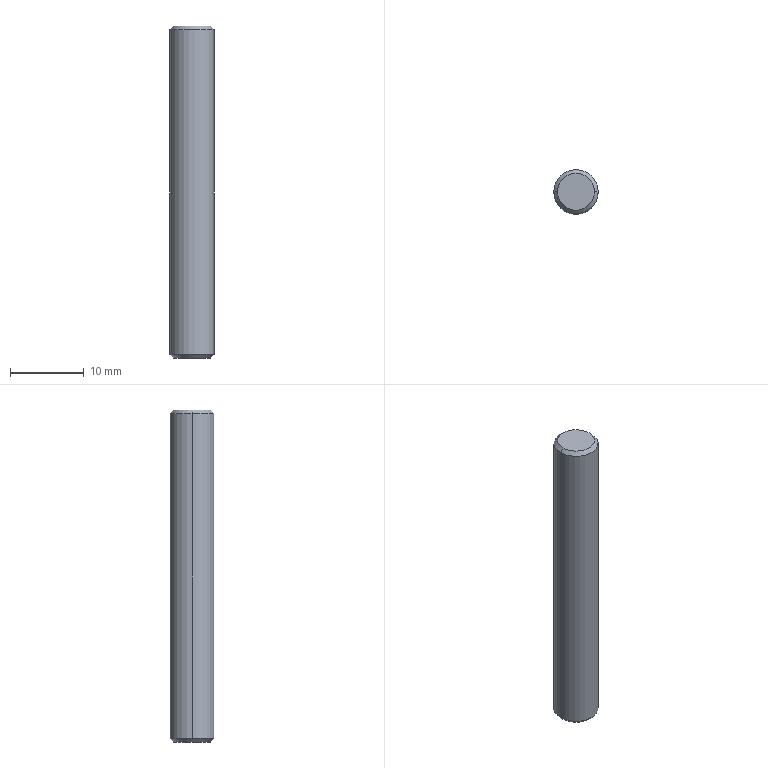Part | SolidWorks | features Chamfer 1, Extrusion 1, HoleWzd 1 | 1 solid | 12 faces | box 6 x 6 x 45 mm | volume 1230 mm3 | cone 6 | cylinder 4 | plane 2 | commonest cylinder face diameters 2.5 x2 6 x2
STEP:
#1=CARTESIAN_POINT('',(-2.5,0.,0.));
#2=VERTEX_POINT('',#1);
#3=CARTESIAN_POINT('',(2.5,0.,0.));
#4=VERTEX_POINT('',#3);
#5=CARTESIAN_POINT('',(0.,0.,0.));
#6=DIRECTION('',(0.,0.,-1.));
#7=DIRECTION('',(1.,0.,0.));
#8=AXIS2_PLACEMENT_3D('',#5,#6,#7);
#9=CIRCLE('',#8,2.5);
#10=EDGE_CURVE('',#2,#4,#9,.T.);
#11=ORIENTED_EDGE('',*,*,#10,.F.);
#12=CARTESIAN_POINT('',(-3.,0.,0.5));
#13=VERTEX_POINT('',#12);
#14=CARTESIAN_POINT('',(-3.,0.,0.5));
#15=DIRECTION('',(-0.7071,0.,0.7071));
#16=VECTOR('',#15,1000.);
#17=LINE('',#14,#16);
#18=EDGE_CURVE('',#2,#13,#17,.T.);
#19=ORIENTED_EDGE('',*,*,#18,.T.);
#20=CARTESIAN_POINT('',(3.,0.,0.5));
#21=VERTEX_POINT('',#20);
#22=CARTESIAN_POINT('',(0.,0.,0.5));
#23=DIRECTION('',(0.,0.,1.));
#24=DIRECTION('',(1.,0.,0.));
#25=AXIS2_PLACEMENT_3D('',#22,#23,#24);
#26=CIRCLE('',#25,3.);
#27=EDGE_CURVE('',#21,#13,#26,.T.);
#28=ORIENTED_EDGE('',*,*,#27,.F.);
#29=CARTESIAN_POINT('',(3.,0.,0.5));
#30=DIRECTION('',(0.7071,0.,0.7071));
#31=VECTOR('',#30,1000.);
#32=LINE('',#29,#31);
#33=EDGE_CURVE('',#4,#21,#32,.T.);
#34=ORIENTED_EDGE('',*,*,#33,.F.);
#35=EDGE_LOOP('',(#11,#19,#28,#34));
#36=FACE_OUTER_BOUND('',#35,.T.);
#37=CARTESIAN_POINT('',(0.,0.,0.5));
#38=DIRECTION('',(0.,0.,1.));
#39=DIRECTION('',(1.,0.,0.));
#40=AXIS2_PLACEMENT_3D('',#37,#38,#39);
#41=CONICAL_SURFACE('',#40,3.,0.7854);
#42=ADVANCED_FACE('',(#36),#41,.T.);
#43=CARTESIAN_POINT('',(2.5,0.,45.));
#44=VERTEX_POINT('',#43);
#45=CARTESIAN_POINT('',(-2.5,0.,45.));
#46=VERTEX_POINT('',#45);
#47=CARTESIAN_POINT('',(0.,0.,45.));
#48=DIRECTION('',(0.,0.,1.));
#49=DIRECTION('',(1.,0.,0.));
#50=AXIS2_PLACEMENT_3D('',#47,#48,#49);
#51=CIRCLE('',#50,2.5);
#52=EDGE_CURVE('',#44,#46,#51,.T.);
#53=ORIENTED_EDGE('',*,*,#52,.F.);
#54=CARTESIAN_POINT('',(3.,0.,44.5));
#55=VERTEX_POINT('',#54);
#56=CARTESIAN_POINT('',(2.5,0.,45.));
#57=DIRECTION('',(0.7071,0.,-0.7071));
#58=VECTOR('',#57,1000.);
#59=LINE('',#56,#58);
#60=EDGE_CURVE('',#44,#55,#59,.T.);
#61=ORIENTED_EDGE('',*,*,#60,.T.);
#62=CARTESIAN_POINT('',(-3.,0.,44.5));
#63=VERTEX_POINT('',#62);
#64=CARTESIAN_POINT('',(0.,0.,44.5));
#65=DIRECTION('',(0.,0.,-1.));
#66=DIRECTION('',(1.,0.,0.));
#67=AXIS2_PLACEMENT_3D('',#64,#65,#66);
#68=CIRCLE('',#67,3.);
#69=EDGE_CURVE('',#63,#55,#68,.T.);
#70=ORIENTED_EDGE('',*,*,#69,.F.);
#71=CARTESIAN_POINT('',(-2.5,0.,45.));
#72=DIRECTION('',(-0.7071,0.,-0.7071));
#73=VECTOR('',#72,1000.);
#74=LINE('',#71,#73);
#75=EDGE_CURVE('',#46,#63,#74,.T.);
#76=ORIENTED_EDGE('',*,*,#75,.F.);
#77=EDGE_LOOP('',(#53,#61,#70,#76));
#78=FACE_OUTER_BOUND('',#77,.T.);
#79=CARTESIAN_POINT('',(0.,0.,45.));
#80=DIRECTION('',(0.,0.,-1.));
#81=DIRECTION('',(-1.,0.,0.));
#82=AXIS2_PLACEMENT_3D('',#79,#80,#81);
#83=CONICAL_SURFACE('',#82,2.5,0.7854);
#84=ADVANCED_FACE('',(#78),#83,.T.);
#85=CARTESIAN_POINT('',(1.25,0.,7.5));
#86=VERTEX_POINT('',#85);
#87=CARTESIAN_POINT('',(-1.25,0.,7.5));
#88=VERTEX_POINT('',#87);
#89=CARTESIAN_POINT('',(0.,0.,7.5));
#90=DIRECTION('',(0.,0.,-1.));
#91=DIRECTION('',(-1.,0.,0.));
#92=AXIS2_PLACEMENT_3D('',#89,#90,#91);
#93=CIRCLE('',#92,1.25);
#94=EDGE_CURVE('',#86,#88,#93,.T.);
#95=ORIENTED_EDGE('',*,*,#94,.F.);
#96=CARTESIAN_POINT('',(1.25,0.,0.));
#97=VERTEX_POINT('',#96);
#98=CARTESIAN_POINT('',(1.25,0.,0.));
#99=DIRECTION('',(0.,0.,-1.));
#100=VECTOR('',#99,1000.);
#101=LINE('',#98,#100);
#102=EDGE_CURVE('',#86,#97,#101,.T.);
#103=ORIENTED_EDGE('',*,*,#102,.T.);
#104=CARTESIAN_POINT('',(-1.25,0.,0.));
#105=VERTEX_POINT('',#104);
#106=CARTESIAN_POINT('',(0.,0.,0.));
#107=DIRECTION('',(0.,0.,-1.));
#108=DIRECTION('',(-1.,0.,0.));
#109=AXIS2_PLACEMENT_3D('',#106,#107,#108);
#110=CIRCLE('',#109,1.25);
#111=EDGE_CURVE('',#97,#105,#110,.T.);
#112=ORIENTED_EDGE('',*,*,#111,.T.);
#113=CARTESIAN_POINT('',(-1.25,0.,0.));
#114=DIRECTION('',(0.,0.,-1.));
#115=VECTOR('',#114,1000.);
#116=LINE('',#113,#115);
#117=EDGE_CURVE('',#88,#105,#116,.T.);
#118=ORIENTED_EDGE('',*,*,#117,.F.);
#119=EDGE_LOOP('',(#95,#103,#112,#118));
#120=FACE_OUTER_BOUND('',#119,.T.);
#121=CARTESIAN_POINT('',(0.,0.,0.));
#122=DIRECTION('',(0.,0.,-1.));
#123=DIRECTION('',(-1.,0.,0.));
#124=AXIS2_PLACEMENT_3D('',#121,#122,#123);
#125=CYLINDRICAL_SURFACE('',#124,1.25);
#126=ADVANCED_FACE('',(#120),#125,.F.);
#127=CARTESIAN_POINT('',(0.,0.,8.251));
#128=VERTEX_POINT('',#127);
#129=CARTESIAN_POINT('',(-1.25,0.,7.5));
#130=DIRECTION('',(-0.8572,0.,-0.515));
#131=VECTOR('',#130,1000.);
#132=LINE('',#129,#131);
#133=EDGE_CURVE('',#128,#88,#132,.T.);
#134=ORIENTED_EDGE('',*,*,#133,.F.);
#135=CARTESIAN_POINT('',(1.25,0.,7.5));
#136=DIRECTION('',(0.8572,0.,-0.515));
#137=VECTOR('',#136,1000.);
#138=LINE('',#135,#137);
#139=EDGE_CURVE('',#128,#86,#138,.T.);
#140=ORIENTED_EDGE('',*,*,#139,.T.);
#141=ORIENTED_EDGE('',*,*,#94,.T.);
#142=EDGE_LOOP('',(#134,#140,#141));
#143=FACE_OUTER_BOUND('',#142,.T.);
#144=CARTESIAN_POINT('',(0.,0.,7.5));
#145=DIRECTION('',(0.,0.,-1.));
#146=DIRECTION('',(-1.,0.,0.));
#147=AXIS2_PLACEMENT_3D('',#144,#145,#146);
#148=CONICAL_SURFACE('',#147,1.25,1.03);
#149=ADVANCED_FACE('',(#143),#148,.F.);
#150=ORIENTED_EDGE('',*,*,#69,.T.);
#151=CARTESIAN_POINT('',(3.,0.,45.));
#152=DIRECTION('',(0.,0.,-1.));
#153=VECTOR('',#152,1000.);
#154=LINE('',#151,#153);
#155=EDGE_CURVE('',#55,#21,#154,.T.);
#156=ORIENTED_EDGE('',*,*,#155,.T.);
#157=ORIENTED_EDGE('',*,*,#27,.T.);
#158=CARTESIAN_POINT('',(-3.,0.,45.));
#159=DIRECTION('',(0.,0.,-1.));
#160=VECTOR('',#159,1000.);
#161=LINE('',#158,#160);
#162=EDGE_CURVE('',#63,#13,#161,.T.);
#163=ORIENTED_EDGE('',*,*,#162,.F.);
#164=EDGE_LOOP('',(#150,#156,#157,#163));
#165=FACE_OUTER_BOUND('',#164,.T.);
#166=CARTESIAN_POINT('',(0.,0.,45.));
#167=DIRECTION('',(0.,0.,-1.));
#168=DIRECTION('',(-1.,0.,0.));
#169=AXIS2_PLACEMENT_3D('',#166,#167,#168);
#170=CYLINDRICAL_SURFACE('',#169,3.);
#171=ADVANCED_FACE('',(#165),#170,.T.);
#172=ORIENTED_EDGE('',*,*,#155,.F.);
#173=CARTESIAN_POINT('',(0.,0.,44.5));
#174=DIRECTION('',(0.,0.,-1.));
#175=DIRECTION('',(1.,0.,0.));
#176=AXIS2_PLACEMENT_3D('',#173,#174,#175);
#177=CIRCLE('',#176,3.);
#178=EDGE_CURVE('',#55,#63,#177,.T.);
#179=ORIENTED_EDGE('',*,*,#178,.T.);
#180=ORIENTED_EDGE('',*,*,#162,.T.);
#181=CARTESIAN_POINT('',(0.,0.,0.5));
#182=DIRECTION('',(0.,0.,1.));
#183=DIRECTION('',(1.,0.,0.));
#184=AXIS2_PLACEMENT_3D('',#181,#182,#183);
#185=CIRCLE('',#184,3.);
#186=EDGE_CURVE('',#13,#21,#185,.T.);
#187=ORIENTED_EDGE('',*,*,#186,.T.);
#188=EDGE_LOOP('',(#172,#179,#180,#187));
#189=FACE_OUTER_BOUND('',#188,.T.);
#190=CARTESIAN_POINT('',(0.,0.,45.));
#191=DIRECTION('',(0.,0.,-1.));
#192=DIRECTION('',(-1.,0.,0.));
#193=AXIS2_PLACEMENT_3D('',#190,#191,#192);
#194=CYLINDRICAL_SURFACE('',#193,3.);
#195=ADVANCED_FACE('',(#189),#194,.T.);
#196=CARTESIAN_POINT('',(0.,0.,45.));
#197=DIRECTION('',(0.,0.,1.));
#198=DIRECTION('',(1.,0.,0.));
#199=AXIS2_PLACEMENT_3D('',#196,#197,#198);
#200=CIRCLE('',#199,2.5);
#201=EDGE_CURVE('',#46,#44,#200,.T.);
#202=ORIENTED_EDGE('',*,*,#201,.T.);
#203=ORIENTED_EDGE('',*,*,#52,.T.);
#204=EDGE_LOOP('',(#202,#203));
#205=FACE_OUTER_BOUND('',#204,.T.);
#206=CARTESIAN_POINT('',(0.,0.,45.));
#207=DIRECTION('',(0.,0.,1.));
#208=DIRECTION('',(1.,0.,0.));
#209=AXIS2_PLACEMENT_3D('',#206,#207,#208);
#210=PLANE('',#209);
#211=ADVANCED_FACE('',(#205),#210,.T.);
#212=CARTESIAN_POINT('',(0.,0.,0.));
#213=DIRECTION('',(0.,0.,-1.));
#214=DIRECTION('',(1.,0.,0.));
#215=AXIS2_PLACEMENT_3D('',#212,#213,#214);
#216=CIRCLE('',#215,2.5);
#217=EDGE_CURVE('',#4,#2,#216,.T.);
#218=ORIENTED_EDGE('',*,*,#217,.T.);
#219=ORIENTED_EDGE('',*,*,#10,.T.);
#220=EDGE_LOOP('',(#218,#219));
#221=FACE_OUTER_BOUND('',#220,.T.);
#222=CARTESIAN_POINT('',(0.,0.,0.));
#223=DIRECTION('',(0.,0.,-1.));
#224=DIRECTION('',(-1.,0.,0.));
#225=AXIS2_PLACEMENT_3D('',#222,#223,#224);
#226=CIRCLE('',#225,1.25);
#227=EDGE_CURVE('',#105,#97,#226,.T.);
#228=ORIENTED_EDGE('',*,*,#227,.F.);
#229=ORIENTED_EDGE('',*,*,#111,.F.);
#230=EDGE_LOOP('',(#228,#229));
#231=FACE_BOUND('',#230,.T.);
#232=CARTESIAN_POINT('',(0.,0.,0.));
#233=DIRECTION('',(0.,0.,1.));
#234=DIRECTION('',(1.,0.,0.));
#235=AXIS2_PLACEMENT_3D('',#232,#233,#234);
#236=PLANE('',#235);
#237=ADVANCED_FACE('',(#221,#231),#236,.F.);
#238=ORIENTED_EDGE('',*,*,#139,.F.);
#239=ORIENTED_EDGE('',*,*,#133,.T.);
#240=CARTESIAN_POINT('',(0.,0.,7.5));
#241=DIRECTION('',(0.,0.,-1.));
#242=DIRECTION('',(-1.,0.,0.));
#243=AXIS2_PLACEMENT_3D('',#240,#241,#242);
#244=CIRCLE('',#243,1.25);
#245=EDGE_CURVE('',#88,#86,#244,.T.);
#246=ORIENTED_EDGE('',*,*,#245,.T.);
#247=EDGE_LOOP('',(#238,#239,#246));
#248=FACE_OUTER_BOUND('',#247,.T.);
#249=CARTESIAN_POINT('',(0.,0.,7.5));
#250=DIRECTION('',(0.,0.,-1.));
#251=DIRECTION('',(-1.,0.,0.));
#252=AXIS2_PLACEMENT_3D('',#249,#250,#251);
#253=CONICAL_SURFACE('',#252,1.25,1.03);
#254=ADVANCED_FACE('',(#248),#253,.F.);
#255=ORIENTED_EDGE('',*,*,#102,.F.);
#256=ORIENTED_EDGE('',*,*,#245,.F.);
#257=ORIENTED_EDGE('',*,*,#117,.T.);
#258=ORIENTED_EDGE('',*,*,#227,.T.);
#259=EDGE_LOOP('',(#255,#256,#257,#258));
#260=FACE_OUTER_BOUND('',#259,.T.);
#261=CARTESIAN_POINT('',(0.,0.,0.));
#262=DIRECTION('',(0.,0.,-1.));
#263=DIRECTION('',(-1.,0.,0.));
#264=AXIS2_PLACEMENT_3D('',#261,#262,#263);
#265=CYLINDRICAL_SURFACE('',#264,1.25);
#266=ADVANCED_FACE('',(#260),#265,.F.);
#267=ORIENTED_EDGE('',*,*,#60,.F.);
#268=ORIENTED_EDGE('',*,*,#201,.F.);
#269=ORIENTED_EDGE('',*,*,#75,.T.);
#270=ORIENTED_EDGE('',*,*,#178,.F.);
#271=EDGE_LOOP('',(#267,#268,#269,#270));
#272=FACE_OUTER_BOUND('',#271,.T.);
#273=CARTESIAN_POINT('',(0.,0.,45.));
#274=DIRECTION('',(0.,0.,-1.));
#275=DIRECTION('',(-1.,0.,0.));
#276=AXIS2_PLACEMENT_3D('',#273,#274,#275);
#277=CONICAL_SURFACE('',#276,2.5,0.7854);
#278=ADVANCED_FACE('',(#272),#277,.T.);
#279=ORIENTED_EDGE('',*,*,#18,.F.);
#280=ORIENTED_EDGE('',*,*,#217,.F.);
#281=ORIENTED_EDGE('',*,*,#33,.T.);
#282=ORIENTED_EDGE('',*,*,#186,.F.);
#283=EDGE_LOOP('',(#279,#280,#281,#282));
#284=FACE_OUTER_BOUND('',#283,.T.);
#285=CARTESIAN_POINT('',(0.,0.,0.5));
#286=DIRECTION('',(0.,0.,1.));
#287=DIRECTION('',(1.,0.,0.));
#288=AXIS2_PLACEMENT_3D('',#285,#286,#287);
#289=CONICAL_SURFACE('',#288,3.,0.7854);
#290=ADVANCED_FACE('',(#284),#289,.T.);
#291=CLOSED_SHELL('',(#42,#84,#126,#149,#171,#195,#211,#237,#254,#266,#278,#290));
#292=MANIFOLD_SOLID_BREP('',#291);
#293=CARTESIAN_POINT('',(0.,0.,0.));
#294=DIRECTION('',(0.,0.,1.));
#295=DIRECTION('',(1.,0.,0.));
#296=AXIS2_PLACEMENT_3D('',#293,#294,#295);
#297=(LENGTH_UNIT()NAMED_UNIT(*)SI_UNIT(.MILLI.,.METRE.));
#298=UNCERTAINTY_MEASURE_WITH_UNIT(LENGTH_MEASURE(0.00001),#297,'','');
#299=(NAMED_UNIT(*)PLANE_ANGLE_UNIT()SI_UNIT($,.RADIAN.));
#300=(NAMED_UNIT(*)SI_UNIT($,.STERADIAN.)SOLID_ANGLE_UNIT());
#301=(GEOMETRIC_REPRESENTATION_CONTEXT(3)GLOBAL_UNCERTAINTY_ASSIGNED_CONTEXT((#298))GLOBAL_UNIT_ASSIGNED_CONTEXT((#297,#299,#300))REPRESENTATION_CONTEXT('',''));
#302=ADVANCED_BREP_SHAPE_REPRESENTATION('',(#292,#296),#301);